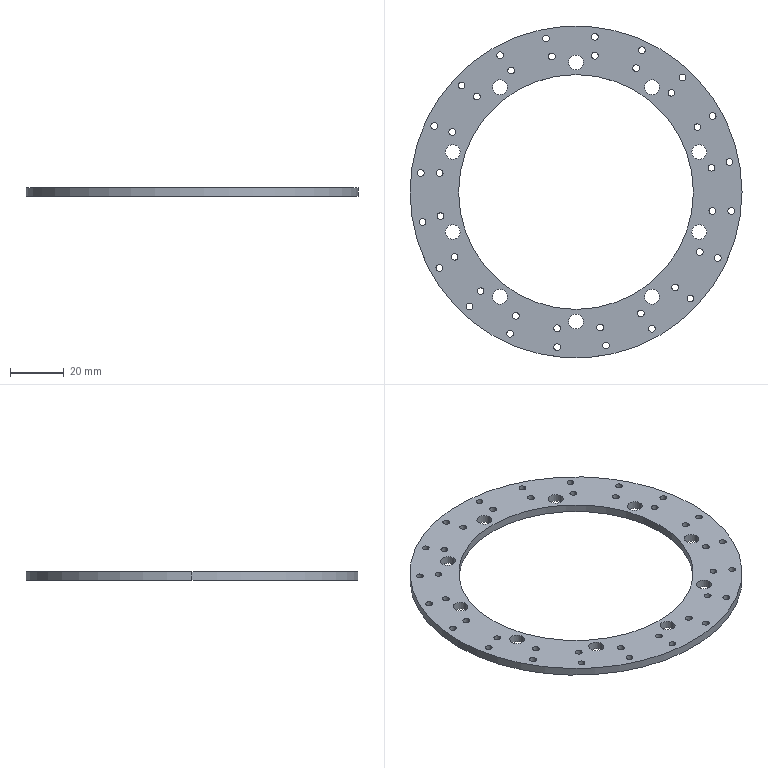Part | SolidWorks | features CirPattern 2, HoleWzd 2, Extrusion 1 | 1 solid | 106 faces | box 123 x 123 x 3 mm | volume 16511 mm3 | cylinder 104 | plane 2 | commonest cylinder face diameters 2.5 x80 5.5 x20 87 x2 123 x2